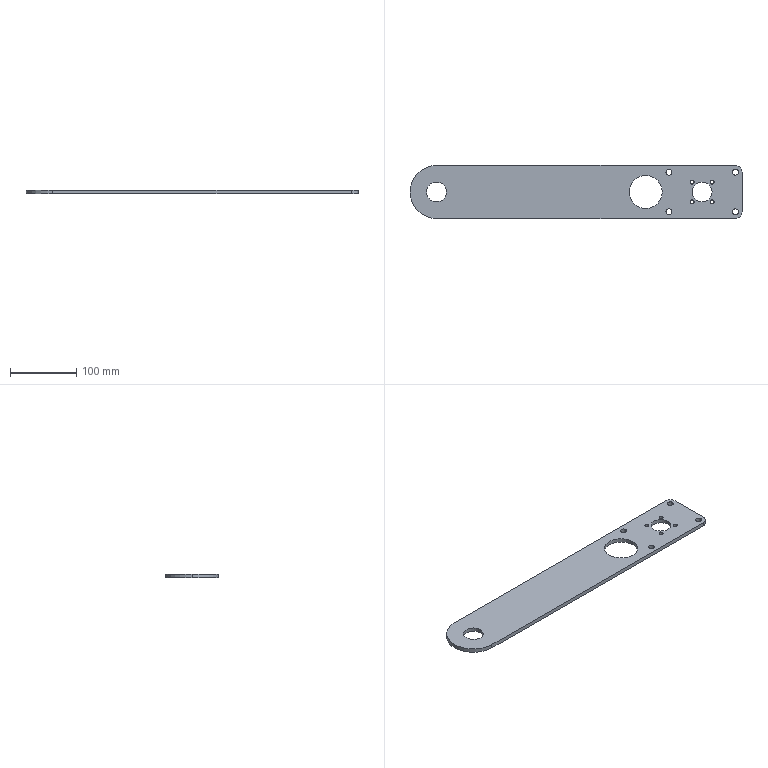Part | STEP file | BCC3 H16_1 | 1 solid | 47 faces | box 500 x 80 x 6 mm | volume 213344 mm3 | cylinder 26 | cone 16 | plane 5 | commonest cylinder face diameters 5 x8 9 x8 30 x4 20 x2 50 x2 80 x2